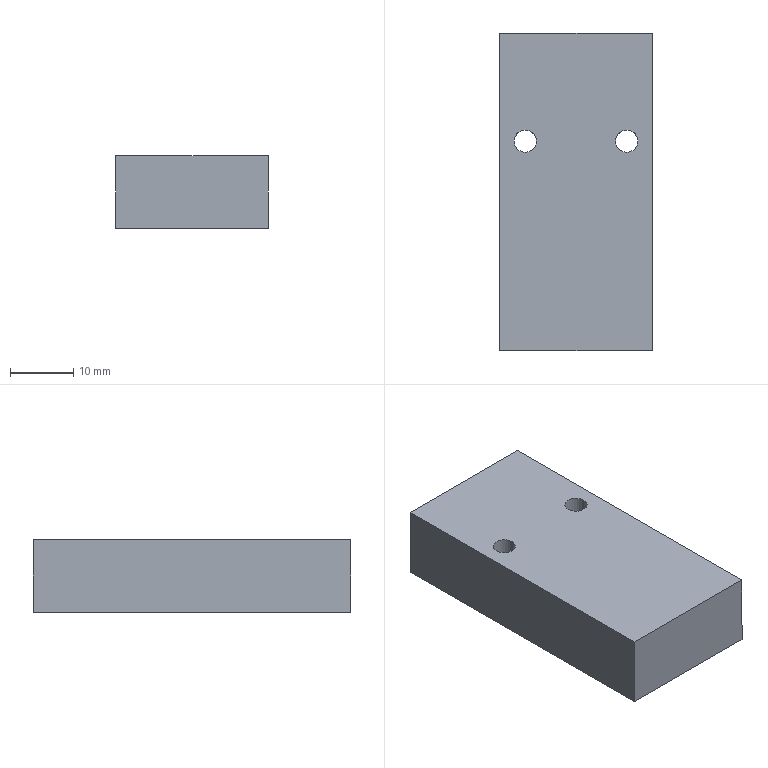Part | SolidWorks | features BaseBody 1 | 1 solid | 10 faces | box 24 x 50 x 11.5 mm | volume 13579 mm3 | plane 6 | cylinder 4 | commonest cylinder face diameters 3.5 x4
STEP:
#1=CARTESIAN_POINT('',(88.874,-120.86,11.5));
#2=VERTEX_POINT('',#1);
#3=CARTESIAN_POINT('',(85.374,-120.86,11.5));
#4=VERTEX_POINT('',#3);
#5=CARTESIAN_POINT('',(87.124,-120.86,11.5));
#6=DIRECTION('',(0.,0.,-1.));
#7=DIRECTION('',(-1.,0.,0.));
#8=AXIS2_PLACEMENT_3D('',#5,#6,#7);
#9=CIRCLE('',#8,1.75);
#10=EDGE_CURVE('',#2,#4,#9,.T.);
#11=ORIENTED_EDGE('',*,*,#10,.F.);
#12=CARTESIAN_POINT('',(88.874,-120.86,0.));
#13=VERTEX_POINT('',#12);
#14=CARTESIAN_POINT('',(88.874,-120.86,56.641));
#15=DIRECTION('',(0.,0.,-1.));
#16=VECTOR('',#15,1000.);
#17=LINE('',#14,#16);
#18=EDGE_CURVE('',#2,#13,#17,.T.);
#19=ORIENTED_EDGE('',*,*,#18,.T.);
#20=CARTESIAN_POINT('',(85.374,-120.86,0.));
#21=VERTEX_POINT('',#20);
#22=CARTESIAN_POINT('',(87.124,-120.86,0.));
#23=DIRECTION('',(0.,0.,1.));
#24=DIRECTION('',(-1.,0.,0.));
#25=AXIS2_PLACEMENT_3D('',#22,#23,#24);
#26=CIRCLE('',#25,1.75);
#27=EDGE_CURVE('',#21,#13,#26,.T.);
#28=ORIENTED_EDGE('',*,*,#27,.F.);
#29=CARTESIAN_POINT('',(85.374,-120.86,56.641));
#30=DIRECTION('',(0.,0.,-1.));
#31=VECTOR('',#30,1000.);
#32=LINE('',#29,#31);
#33=EDGE_CURVE('',#4,#21,#32,.T.);
#34=ORIENTED_EDGE('',*,*,#33,.F.);
#35=EDGE_LOOP('',(#11,#19,#28,#34));
#36=FACE_OUTER_BOUND('',#35,.T.);
#37=CARTESIAN_POINT('',(87.124,-120.86,56.641));
#38=DIRECTION('',(0.,0.,-1.));
#39=DIRECTION('',(-1.,0.,0.));
#40=AXIS2_PLACEMENT_3D('',#37,#38,#39);
#41=CYLINDRICAL_SURFACE('',#40,1.75);
#42=ADVANCED_FACE('',(#36),#41,.F.);
#43=CARTESIAN_POINT('',(104.874,-120.86,11.5));
#44=VERTEX_POINT('',#43);
#45=CARTESIAN_POINT('',(101.374,-120.86,11.5));
#46=VERTEX_POINT('',#45);
#47=CARTESIAN_POINT('',(103.124,-120.86,11.5));
#48=DIRECTION('',(0.,0.,-1.));
#49=DIRECTION('',(-1.,0.,0.));
#50=AXIS2_PLACEMENT_3D('',#47,#48,#49);
#51=CIRCLE('',#50,1.75);
#52=EDGE_CURVE('',#44,#46,#51,.T.);
#53=ORIENTED_EDGE('',*,*,#52,.F.);
#54=CARTESIAN_POINT('',(104.874,-120.86,0.));
#55=VERTEX_POINT('',#54);
#56=CARTESIAN_POINT('',(104.874,-120.86,56.641));
#57=DIRECTION('',(0.,0.,-1.));
#58=VECTOR('',#57,1000.);
#59=LINE('',#56,#58);
#60=EDGE_CURVE('',#44,#55,#59,.T.);
#61=ORIENTED_EDGE('',*,*,#60,.T.);
#62=CARTESIAN_POINT('',(101.374,-120.86,0.));
#63=VERTEX_POINT('',#62);
#64=CARTESIAN_POINT('',(103.124,-120.86,0.));
#65=DIRECTION('',(0.,0.,1.));
#66=DIRECTION('',(-1.,0.,0.));
#67=AXIS2_PLACEMENT_3D('',#64,#65,#66);
#68=CIRCLE('',#67,1.75);
#69=EDGE_CURVE('',#63,#55,#68,.T.);
#70=ORIENTED_EDGE('',*,*,#69,.F.);
#71=CARTESIAN_POINT('',(101.374,-120.86,56.641));
#72=DIRECTION('',(0.,0.,-1.));
#73=VECTOR('',#72,1000.);
#74=LINE('',#71,#73);
#75=EDGE_CURVE('',#46,#63,#74,.T.);
#76=ORIENTED_EDGE('',*,*,#75,.F.);
#77=EDGE_LOOP('',(#53,#61,#70,#76));
#78=FACE_OUTER_BOUND('',#77,.T.);
#79=CARTESIAN_POINT('',(103.124,-120.86,56.641));
#80=DIRECTION('',(0.,0.,-1.));
#81=DIRECTION('',(-1.,0.,0.));
#82=AXIS2_PLACEMENT_3D('',#79,#80,#81);
#83=CYLINDRICAL_SURFACE('',#82,1.75);
#84=ADVANCED_FACE('',(#78),#83,.F.);
#85=CARTESIAN_POINT('',(87.124,-120.86,11.5));
#86=DIRECTION('',(0.,0.,-1.));
#87=DIRECTION('',(-1.,0.,0.));
#88=AXIS2_PLACEMENT_3D('',#85,#86,#87);
#89=CIRCLE('',#88,1.75);
#90=EDGE_CURVE('',#4,#2,#89,.T.);
#91=ORIENTED_EDGE('',*,*,#90,.T.);
#92=ORIENTED_EDGE('',*,*,#10,.T.);
#93=EDGE_LOOP('',(#91,#92));
#94=FACE_BOUND('',#93,.T.);
#95=CARTESIAN_POINT('',(103.124,-120.86,11.5));
#96=DIRECTION('',(0.,0.,-1.));
#97=DIRECTION('',(-1.,0.,0.));
#98=AXIS2_PLACEMENT_3D('',#95,#96,#97);
#99=CIRCLE('',#98,1.75);
#100=EDGE_CURVE('',#46,#44,#99,.T.);
#101=ORIENTED_EDGE('',*,*,#100,.T.);
#102=ORIENTED_EDGE('',*,*,#52,.T.);
#103=EDGE_LOOP('',(#101,#102));
#104=FACE_BOUND('',#103,.T.);
#105=CARTESIAN_POINT('',(83.124,-103.86,11.5));
#106=VERTEX_POINT('',#105);
#107=CARTESIAN_POINT('',(83.124,-153.86,11.5));
#108=VERTEX_POINT('',#107);
#109=CARTESIAN_POINT('',(83.124,-128.86,11.5));
#110=DIRECTION('',(0.,-1.,0.));
#111=VECTOR('',#110,1000.);
#112=LINE('',#109,#111);
#113=EDGE_CURVE('',#106,#108,#112,.T.);
#114=ORIENTED_EDGE('',*,*,#113,.T.);
#115=CARTESIAN_POINT('',(107.124,-153.86,11.5));
#116=VERTEX_POINT('',#115);
#117=CARTESIAN_POINT('',(95.124,-153.86,11.5));
#118=DIRECTION('',(1.,0.,0.));
#119=VECTOR('',#118,1000.);
#120=LINE('',#117,#119);
#121=EDGE_CURVE('',#108,#116,#120,.T.);
#122=ORIENTED_EDGE('',*,*,#121,.T.);
#123=CARTESIAN_POINT('',(107.124,-103.86,11.5));
#124=VERTEX_POINT('',#123);
#125=CARTESIAN_POINT('',(107.124,-128.86,11.5));
#126=DIRECTION('',(0.,1.,0.));
#127=VECTOR('',#126,1000.);
#128=LINE('',#125,#127);
#129=EDGE_CURVE('',#116,#124,#128,.T.);
#130=ORIENTED_EDGE('',*,*,#129,.T.);
#131=CARTESIAN_POINT('',(95.124,-103.86,11.5));
#132=DIRECTION('',(-1.,0.,0.));
#133=VECTOR('',#132,1000.);
#134=LINE('',#131,#133);
#135=EDGE_CURVE('',#124,#106,#134,.T.);
#136=ORIENTED_EDGE('',*,*,#135,.T.);
#137=EDGE_LOOP('',(#114,#122,#130,#136));
#138=FACE_OUTER_BOUND('',#137,.T.);
#139=CARTESIAN_POINT('',(95.124,-128.86,11.5));
#140=DIRECTION('',(0.,0.,1.));
#141=DIRECTION('',(1.,0.,0.));
#142=AXIS2_PLACEMENT_3D('',#139,#140,#141);
#143=PLANE('',#142);
#144=ADVANCED_FACE('',(#94,#104,#138),#143,.T.);
#145=ORIENTED_EDGE('',*,*,#18,.F.);
#146=ORIENTED_EDGE('',*,*,#90,.F.);
#147=ORIENTED_EDGE('',*,*,#33,.T.);
#148=CARTESIAN_POINT('',(87.124,-120.86,0.));
#149=DIRECTION('',(0.,0.,1.));
#150=DIRECTION('',(-1.,0.,0.));
#151=AXIS2_PLACEMENT_3D('',#148,#149,#150);
#152=CIRCLE('',#151,1.75);
#153=EDGE_CURVE('',#13,#21,#152,.T.);
#154=ORIENTED_EDGE('',*,*,#153,.F.);
#155=EDGE_LOOP('',(#145,#146,#147,#154));
#156=FACE_OUTER_BOUND('',#155,.T.);
#157=CARTESIAN_POINT('',(87.124,-120.86,56.641));
#158=DIRECTION('',(0.,0.,-1.));
#159=DIRECTION('',(-1.,0.,0.));
#160=AXIS2_PLACEMENT_3D('',#157,#158,#159);
#161=CYLINDRICAL_SURFACE('',#160,1.75);
#162=ADVANCED_FACE('',(#156),#161,.F.);
#163=ORIENTED_EDGE('',*,*,#60,.F.);
#164=ORIENTED_EDGE('',*,*,#100,.F.);
#165=ORIENTED_EDGE('',*,*,#75,.T.);
#166=CARTESIAN_POINT('',(103.124,-120.86,0.));
#167=DIRECTION('',(0.,0.,1.));
#168=DIRECTION('',(-1.,0.,0.));
#169=AXIS2_PLACEMENT_3D('',#166,#167,#168);
#170=CIRCLE('',#169,1.75);
#171=EDGE_CURVE('',#55,#63,#170,.T.);
#172=ORIENTED_EDGE('',*,*,#171,.F.);
#173=EDGE_LOOP('',(#163,#164,#165,#172));
#174=FACE_OUTER_BOUND('',#173,.T.);
#175=CARTESIAN_POINT('',(103.124,-120.86,56.641));
#176=DIRECTION('',(0.,0.,-1.));
#177=DIRECTION('',(-1.,0.,0.));
#178=AXIS2_PLACEMENT_3D('',#175,#176,#177);
#179=CYLINDRICAL_SURFACE('',#178,1.75);
#180=ADVANCED_FACE('',(#174),#179,.F.);
#181=CARTESIAN_POINT('',(83.124,-153.86,0.));
#182=VERTEX_POINT('',#181);
#183=CARTESIAN_POINT('',(107.124,-153.86,0.));
#184=VERTEX_POINT('',#183);
#185=CARTESIAN_POINT('',(107.124,-153.86,0.));
#186=DIRECTION('',(1.,0.,0.));
#187=VECTOR('',#186,1000.);
#188=LINE('',#185,#187);
#189=EDGE_CURVE('',#182,#184,#188,.T.);
#190=ORIENTED_EDGE('',*,*,#189,.T.);
#191=CARTESIAN_POINT('',(107.124,-153.86,0.));
#192=DIRECTION('',(0.,0.,1.));
#193=VECTOR('',#192,1000.);
#194=LINE('',#191,#193);
#195=EDGE_CURVE('',#184,#116,#194,.T.);
#196=ORIENTED_EDGE('',*,*,#195,.T.);
#197=ORIENTED_EDGE('',*,*,#121,.F.);
#198=CARTESIAN_POINT('',(83.124,-153.86,0.));
#199=DIRECTION('',(0.,0.,-1.));
#200=VECTOR('',#199,1000.);
#201=LINE('',#198,#200);
#202=EDGE_CURVE('',#108,#182,#201,.T.);
#203=ORIENTED_EDGE('',*,*,#202,.T.);
#204=EDGE_LOOP('',(#190,#196,#197,#203));
#205=FACE_OUTER_BOUND('',#204,.T.);
#206=CARTESIAN_POINT('',(107.124,-153.86,0.));
#207=DIRECTION('',(0.,-1.,0.));
#208=DIRECTION('',(0.,0.,-1.));
#209=AXIS2_PLACEMENT_3D('',#206,#207,#208);
#210=PLANE('',#209);
#211=ADVANCED_FACE('',(#205),#210,.T.);
#212=CARTESIAN_POINT('',(83.124,-103.86,0.));
#213=VERTEX_POINT('',#212);
#214=CARTESIAN_POINT('',(83.124,-153.86,0.));
#215=DIRECTION('',(0.,-1.,0.));
#216=VECTOR('',#215,1000.);
#217=LINE('',#214,#216);
#218=EDGE_CURVE('',#213,#182,#217,.T.);
#219=ORIENTED_EDGE('',*,*,#218,.T.);
#220=ORIENTED_EDGE('',*,*,#202,.F.);
#221=ORIENTED_EDGE('',*,*,#113,.F.);
#222=CARTESIAN_POINT('',(83.124,-103.86,0.));
#223=DIRECTION('',(0.,0.,-1.));
#224=VECTOR('',#223,1000.);
#225=LINE('',#222,#224);
#226=EDGE_CURVE('',#106,#213,#225,.T.);
#227=ORIENTED_EDGE('',*,*,#226,.T.);
#228=EDGE_LOOP('',(#219,#220,#221,#227));
#229=FACE_OUTER_BOUND('',#228,.T.);
#230=CARTESIAN_POINT('',(83.124,-153.86,0.));
#231=DIRECTION('',(-1.,0.,0.));
#232=DIRECTION('',(0.,0.,1.));
#233=AXIS2_PLACEMENT_3D('',#230,#231,#232);
#234=PLANE('',#233);
#235=ADVANCED_FACE('',(#229),#234,.T.);
#236=CARTESIAN_POINT('',(107.124,-103.86,0.));
#237=VERTEX_POINT('',#236);
#238=CARTESIAN_POINT('',(83.124,-103.86,0.));
#239=DIRECTION('',(-1.,0.,0.));
#240=VECTOR('',#239,1000.);
#241=LINE('',#238,#240);
#242=EDGE_CURVE('',#237,#213,#241,.T.);
#243=ORIENTED_EDGE('',*,*,#242,.T.);
#244=ORIENTED_EDGE('',*,*,#226,.F.);
#245=ORIENTED_EDGE('',*,*,#135,.F.);
#246=CARTESIAN_POINT('',(107.124,-103.86,0.));
#247=DIRECTION('',(0.,0.,-1.));
#248=VECTOR('',#247,1000.);
#249=LINE('',#246,#248);
#250=EDGE_CURVE('',#124,#237,#249,.T.);
#251=ORIENTED_EDGE('',*,*,#250,.T.);
#252=EDGE_LOOP('',(#243,#244,#245,#251));
#253=FACE_OUTER_BOUND('',#252,.T.);
#254=CARTESIAN_POINT('',(83.124,-103.86,0.));
#255=DIRECTION('',(0.,1.,0.));
#256=DIRECTION('',(0.,0.,1.));
#257=AXIS2_PLACEMENT_3D('',#254,#255,#256);
#258=PLANE('',#257);
#259=ADVANCED_FACE('',(#253),#258,.T.);
#260=CARTESIAN_POINT('',(107.124,-103.86,0.));
#261=DIRECTION('',(0.,1.,0.));
#262=VECTOR('',#261,1000.);
#263=LINE('',#260,#262);
#264=EDGE_CURVE('',#184,#237,#263,.T.);
#265=ORIENTED_EDGE('',*,*,#264,.T.);
#266=ORIENTED_EDGE('',*,*,#250,.F.);
#267=ORIENTED_EDGE('',*,*,#129,.F.);
#268=ORIENTED_EDGE('',*,*,#195,.F.);
#269=EDGE_LOOP('',(#265,#266,#267,#268));
#270=FACE_OUTER_BOUND('',#269,.T.);
#271=CARTESIAN_POINT('',(107.124,-103.86,0.));
#272=DIRECTION('',(1.,0.,0.));
#273=DIRECTION('',(0.,0.,-1.));
#274=AXIS2_PLACEMENT_3D('',#271,#272,#273);
#275=PLANE('',#274);
#276=ADVANCED_FACE('',(#270),#275,.T.);
#277=ORIENTED_EDGE('',*,*,#27,.T.);
#278=ORIENTED_EDGE('',*,*,#153,.T.);
#279=EDGE_LOOP('',(#277,#278));
#280=FACE_BOUND('',#279,.T.);
#281=ORIENTED_EDGE('',*,*,#69,.T.);
#282=ORIENTED_EDGE('',*,*,#171,.T.);
#283=EDGE_LOOP('',(#281,#282));
#284=FACE_BOUND('',#283,.T.);
#285=ORIENTED_EDGE('',*,*,#264,.F.);
#286=ORIENTED_EDGE('',*,*,#189,.F.);
#287=ORIENTED_EDGE('',*,*,#218,.F.);
#288=ORIENTED_EDGE('',*,*,#242,.F.);
#289=EDGE_LOOP('',(#285,#286,#287,#288));
#290=FACE_OUTER_BOUND('',#289,.T.);
#291=CARTESIAN_POINT('',(95.124,-128.86,0.));
#292=DIRECTION('',(0.,0.,1.));
#293=DIRECTION('',(1.,0.,0.));
#294=AXIS2_PLACEMENT_3D('',#291,#292,#293);
#295=PLANE('',#294);
#296=ADVANCED_FACE('',(#280,#284,#290),#295,.F.);
#297=CLOSED_SHELL('',(#42,#84,#144,#162,#180,#211,#235,#259,#276,#296));
#298=MANIFOLD_SOLID_BREP('',#297);
#299=CARTESIAN_POINT('',(0.,0.,0.));
#300=DIRECTION('',(0.,0.,1.));
#301=DIRECTION('',(1.,0.,0.));
#302=AXIS2_PLACEMENT_3D('',#299,#300,#301);
#303=(LENGTH_UNIT()NAMED_UNIT(*)SI_UNIT(.MILLI.,.METRE.));
#304=UNCERTAINTY_MEASURE_WITH_UNIT(LENGTH_MEASURE(0.00001),#303,'','');
#305=(NAMED_UNIT(*)PLANE_ANGLE_UNIT()SI_UNIT($,.RADIAN.));
#306=(NAMED_UNIT(*)SI_UNIT($,.STERADIAN.)SOLID_ANGLE_UNIT());
#307=(GEOMETRIC_REPRESENTATION_CONTEXT(3)GLOBAL_UNCERTAINTY_ASSIGNED_CONTEXT((#304))GLOBAL_UNIT_ASSIGNED_CONTEXT((#303,#305,#306))REPRESENTATION_CONTEXT('',''));
#308=ADVANCED_BREP_SHAPE_REPRESENTATION('',(#298,#302),#307);